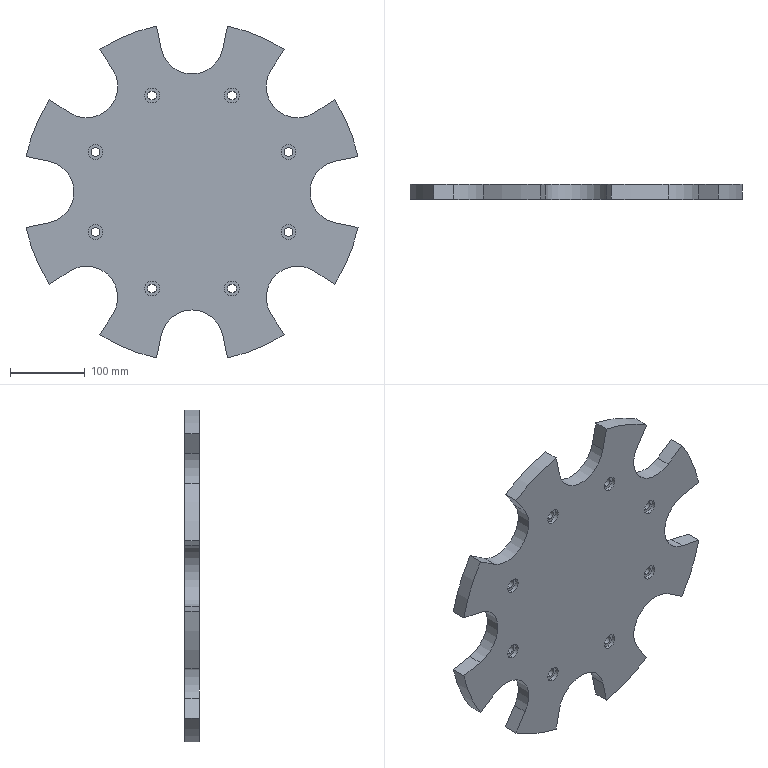Part | SolidWorks | features BaseBody 1 | 1 solid | 77 faces | box 444.972 x 20 x 444.972 mm | volume 2405585 mm3 | cylinder 51 | plane 26 | commonest cylinder face diameters 12 x16 20 x16 84 x11 455 x8